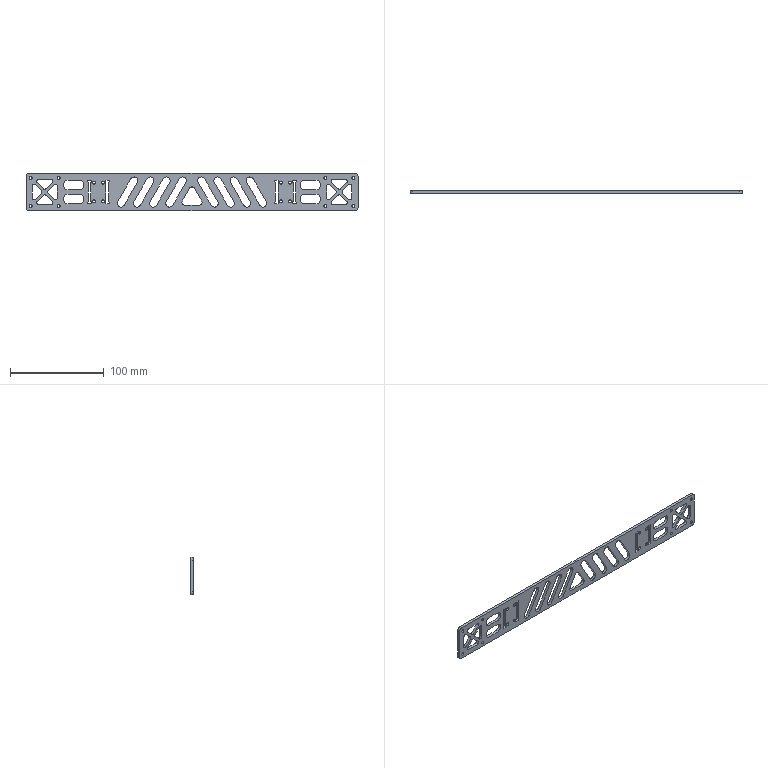Part | SolidWorks | features ICE 3, Extrusion 1, Fillet 1 | 1 solid | 206 faces | box 355 x 3 x 40 mm | volume 28604 mm3 | cylinder 133 | plane 73 | commonest cylinder face diameters 4 x46 3.2 x32 8 x24 1.5 x16 10 x8 6 x7